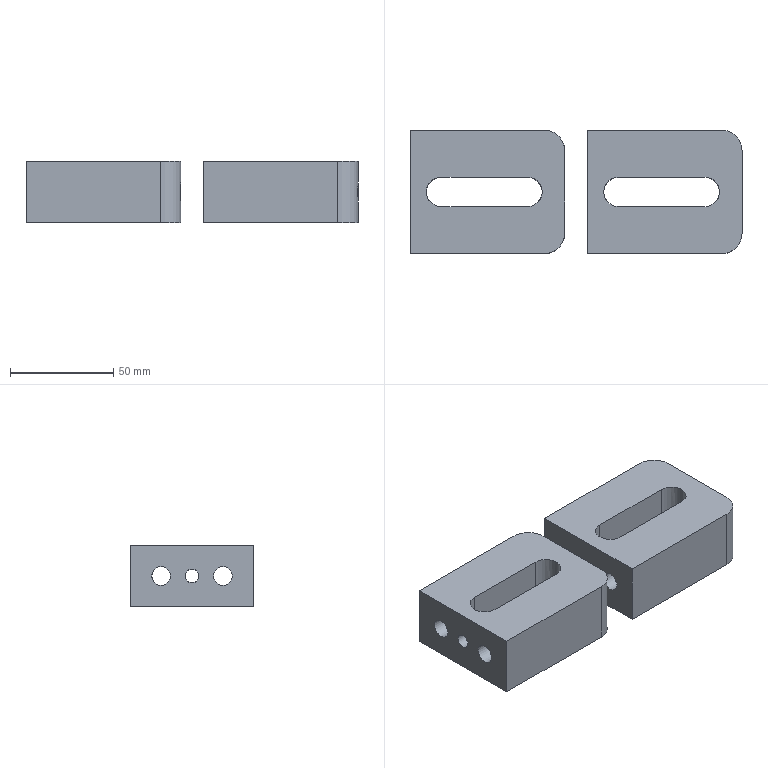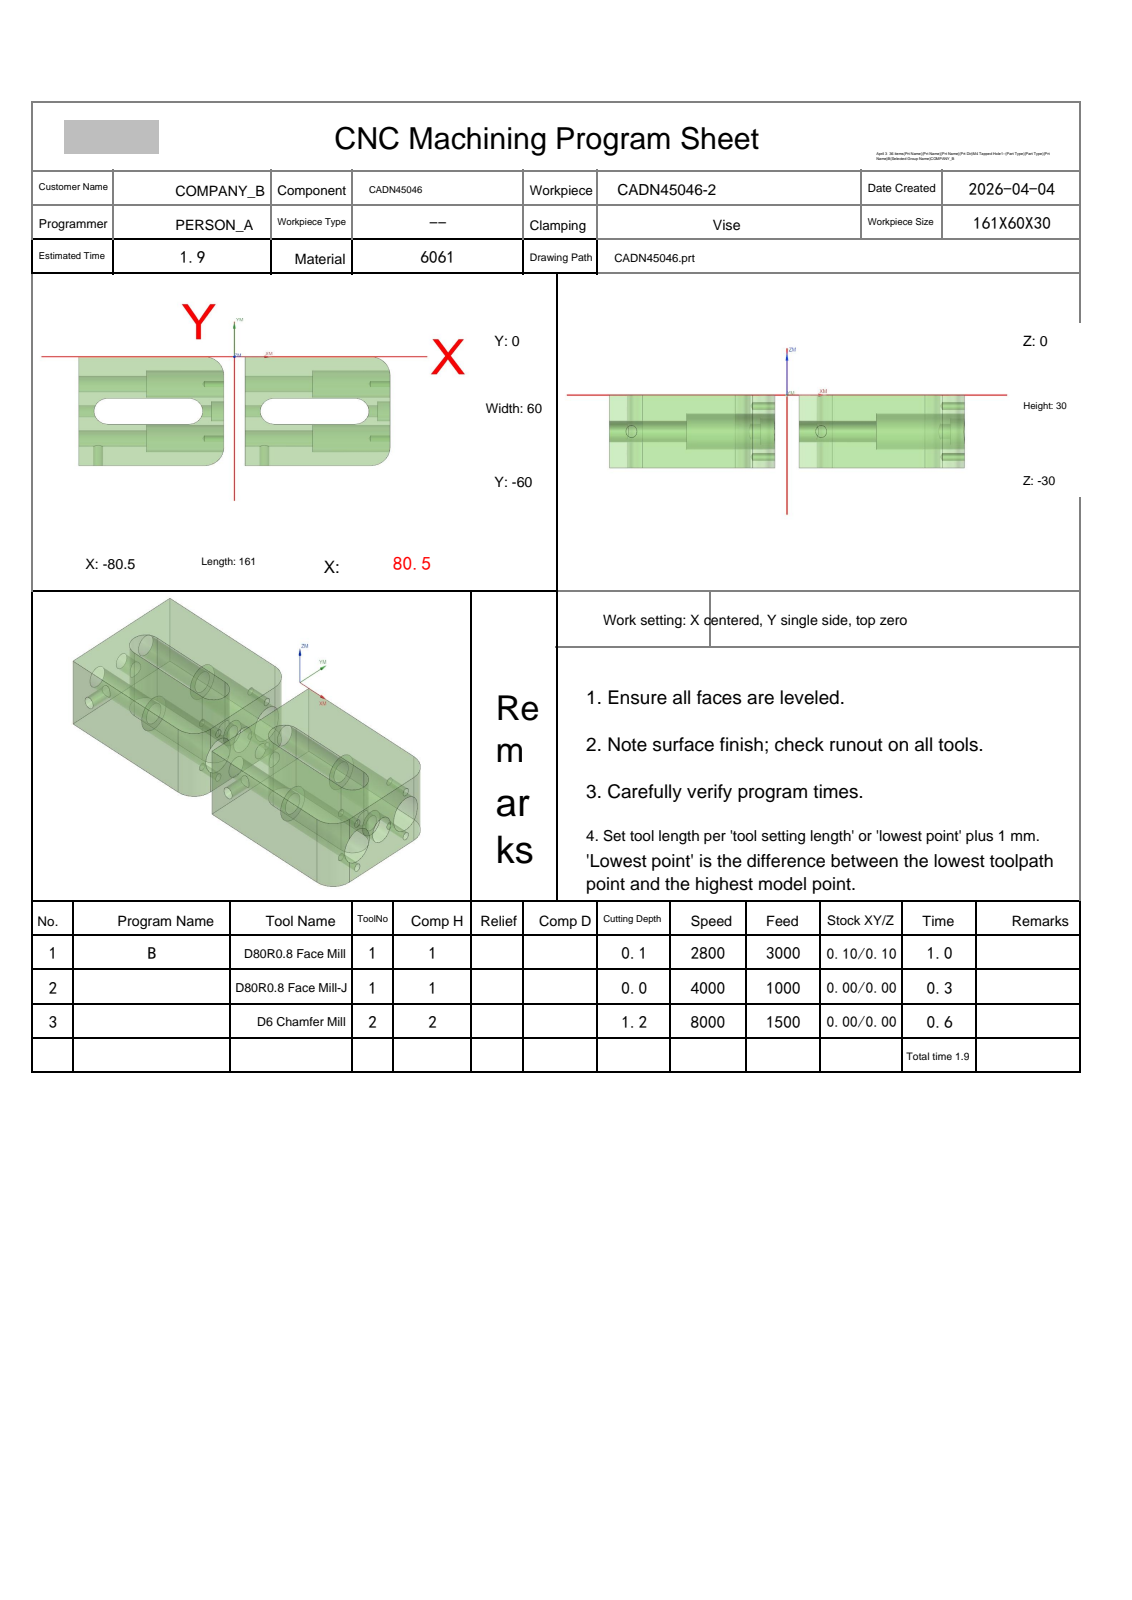NC program | NX | posted by the shop | part box 161 x 60 x 30 mm
Whole program:
%
O0001
(Machine time: 2.42 MIN)
(===Total Tool:2===)
(T1=D80R0.8 Face Mill D=80.  R=0.8  D-  H01 Z=0.    )
(T2=D6 Chamfer Mill   D=6.   R=0.   D-  H02 Z=-1.2  )
G80 G90 G17 G49 G40
G91 G28 Z0
M01
N1 T01 M06
(D80R0.8 Face Mill  D=80. R=0.8 H=01 ce=0.10 di=0.10)
G00 G90 G54 X132.597 Y-30. M03 S2800
G43 H01 Z20.
M08
Z6.011
G01 Z4.011 F3000.
X120.597
X-120.597
X-132.597
Z6.011
G00 X132.597
Z5.522
G01 Z3.522
X120.597
X-120.597
X-132.597
Z5.522
G00 X132.597
Z5.033
G01 Z3.033
X120.597
X-120.597
X-132.597
Z5.033
G00 X132.597
Z4.544
G01 Z2.544
X120.597
X-120.597
X-132.597
Z4.544
G00 Z20.
X132.597
Z4.056
G01 Z2.056
X120.597
X-120.597
X-132.597
Z4.056
G00 Z20.
X132.597
Z3.567
G01 Z1.567
X120.597
X-120.597
X-132.597
Z3.567
G00 Z20.
X132.597
Z3.078
G01 Z1.078
X120.597
X-120.597
X-132.597
Z3.078
G00 Z20.
X132.597
Z2.589
G01 Z.589
X120.597
X-120.597
X-132.597
Z2.589
G00 Z20.
X132.597
Z2.1
G01 Z.1
X120.597
X-120.597
X-132.597
Z2.1
G00 Z20.
G91 G28 Z0.0
M05
M09
G91 G28 Z0.0
M01
N2 T01 M06
(D80R0.8 Face Mill-J  D=80. R=0.8 H=01 ce=0.00 di=0.00)
G00 G90 G54 X132.499 Y-30. M03 S4000
G43 H01 Z20.
M08
Z2.
G01 Z0.0 F1000.
X120.499
X-120.499
X-132.499
Z2.
G00 Z20.
G91 G28 Z0.0
M05
M09
G91 G28 Z0.0
M01
N3 T02 M06
(D6 Chamfer Mill  D=6. R=0. H=02 ce=0.00 di=0.00)
G00 G90 G54 X37.614 Y1.127 M03 S8000
G43 H02 Z20.
M08
Z.272
G01 Z-1.2 F1350.
G03 X37.9 Y.927 I1.286 J1.532
G01 X37.946 Y.897
X38. Y.9
X70.5 F1500.
G02 X81.4 Y-10. I0.0 J-10.9
G01 Y-50.
G02 X70.5 Y-60.9 I-10.9 J0.0
G01 X5.5
G02 X4.6 Y-60. I0.0 J.9
G01 Y0.0
G02 X5.5 Y.9 I.9 J0.0
G01 X38.
X38.054 Y.897
X38.1 Y.927
G03 X38.386 Y1.127 I-1. J1.732
G01 Z.272
G00 Z10.
X41.886 Y-24.027
Z.272
G01 Z-1.2 F1350.
G03 X41.6 Y-23.827 I-1.286 J-1.532
G01 X41.554 Y-23.797
X41.5 Y-23.8
X20.5 F1500.
G03 X14.3 Y-30. I0.0 J-6.2
X20.5 Y-36.2 I6.2 J0.0
G01 X62.5
G03 X68.7 Y-30. I0.0 J6.2
X62.5 Y-23.8 I-6.2 J0.0
G01 X41.5
X41.446 Y-23.797
X41.4 Y-23.827
G03 X41.114 Y-24.027 I1. J-1.732
G01 Z.272
G00 Z10.
X-81.627 Y-30.386
Z.272
G01 Z-1.2 F1350.
G03 X-81.427 Y-30.1 I-1.532 J1.286
G01 X-81.397 Y-30.054
X-81.4 Y-30.
Y0.0 F1500.
G02 X-80.5 Y.9 I.9 J0.0
G01 X-15.5
G02 X-4.6 Y-10. I0.0 J-10.9
G01 Y-50.
G02 X-15.5 Y-60.9 I-10.9 J0.0
G01 X-80.5
G02 X-81.4 Y-60. I0.0 J.9
G01 Y-30.
X-81.397 Y-29.946
X-81.427 Y-29.9
G03 X-81.627 Y-29.614 I-1.732 J-1.
G01 Z.272
G00 Z10.
X-44.886 Y-35.973
Z.272
G01 Z-1.2 F1350.
G03 X-44.6 Y-36.173 I1.286 J1.532
G01 X-44.554 Y-36.203
X-44.5 Y-36.2
X-23.5 F1500.
G03 X-17.3 Y-30. I0.0 J6.2
X-23.5 Y-23.8 I-6.2 J0.0
G01 X-65.5
G03 X-71.7 Y-30. I0.0 J-6.2
X-65.5 Y-36.2 I6.2 J0.0
G01 X-44.5
X-44.446 Y-36.203
X-44.4 Y-36.173
G03 X-44.114 Y-35.973 I-1. J1.732
G01 Z.272
G00 Z20.
M05
M09
G91 G28 Z0.0
G91 G28 Y0.0
M30
%